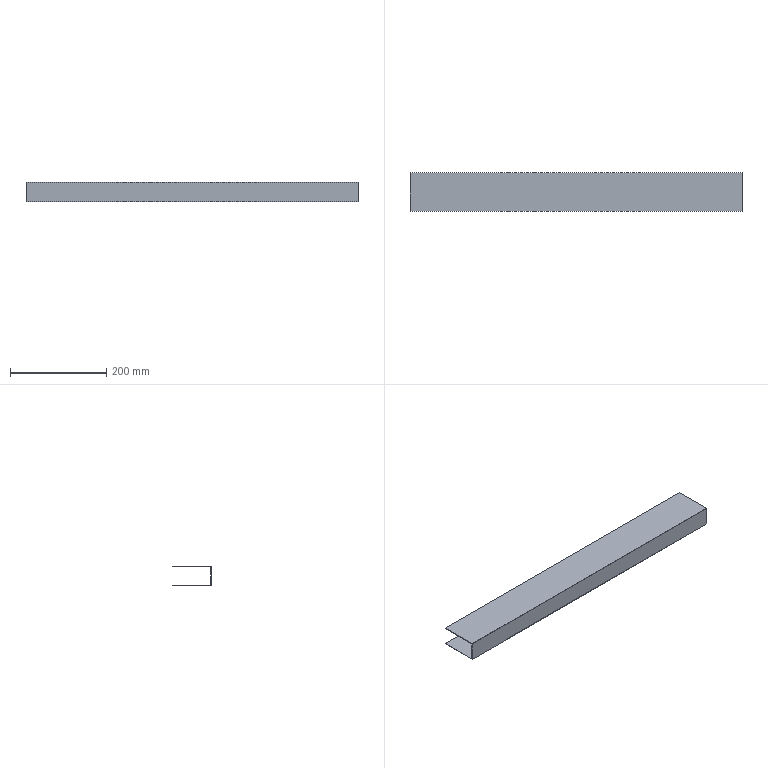Part | SolidWorks | features BaseBody 1 | 1 solid | 10 faces | box 690 x 80 x 40 mm | volume 136620 mm3 | plane 10
STEP:
#1=CARTESIAN_POINT('',(0.,1.,19.));
#2=VERTEX_POINT('',#1);
#3=CARTESIAN_POINT('',(0.,80.,19.));
#4=VERTEX_POINT('',#3);
#5=CARTESIAN_POINT('',(0.,0.,19.));
#6=DIRECTION('',(0.,1.,0.));
#7=VECTOR('',#6,1000.);
#8=LINE('',#5,#7);
#9=EDGE_CURVE('',#2,#4,#8,.T.);
#10=ORIENTED_EDGE('',*,*,#9,.F.);
#11=CARTESIAN_POINT('',(0.,1.,-19.));
#12=VERTEX_POINT('',#11);
#13=CARTESIAN_POINT('',(0.,1.,20.));
#14=DIRECTION('',(0.,0.,1.));
#15=VECTOR('',#14,1000.);
#16=LINE('',#13,#15);
#17=EDGE_CURVE('',#12,#2,#16,.T.);
#18=ORIENTED_EDGE('',*,*,#17,.F.);
#19=CARTESIAN_POINT('',(0.,80.,-19.));
#20=VERTEX_POINT('',#19);
#21=CARTESIAN_POINT('',(0.,0.,-19.));
#22=DIRECTION('',(0.,-1.,0.));
#23=VECTOR('',#22,1000.);
#24=LINE('',#21,#23);
#25=EDGE_CURVE('',#20,#12,#24,.T.);
#26=ORIENTED_EDGE('',*,*,#25,.F.);
#27=CARTESIAN_POINT('',(0.,80.,-20.));
#28=VERTEX_POINT('',#27);
#29=CARTESIAN_POINT('',(0.,80.,-19.));
#30=DIRECTION('',(0.,0.,-1.));
#31=VECTOR('',#30,1000.);
#32=LINE('',#29,#31);
#33=EDGE_CURVE('',#20,#28,#32,.T.);
#34=ORIENTED_EDGE('',*,*,#33,.T.);
#35=CARTESIAN_POINT('',(0.,0.,-20.));
#36=VERTEX_POINT('',#35);
#37=CARTESIAN_POINT('',(0.,0.,-20.));
#38=DIRECTION('',(0.,-1.,0.));
#39=VECTOR('',#38,1000.);
#40=LINE('',#37,#39);
#41=EDGE_CURVE('',#28,#36,#40,.T.);
#42=ORIENTED_EDGE('',*,*,#41,.T.);
#43=CARTESIAN_POINT('',(0.,0.,20.));
#44=VERTEX_POINT('',#43);
#45=CARTESIAN_POINT('',(0.,0.,20.));
#46=DIRECTION('',(0.,0.,1.));
#47=VECTOR('',#46,1000.);
#48=LINE('',#45,#47);
#49=EDGE_CURVE('',#36,#44,#48,.T.);
#50=ORIENTED_EDGE('',*,*,#49,.T.);
#51=CARTESIAN_POINT('',(0.,80.,20.));
#52=VERTEX_POINT('',#51);
#53=CARTESIAN_POINT('',(0.,0.,20.));
#54=DIRECTION('',(0.,1.,0.));
#55=VECTOR('',#54,1000.);
#56=LINE('',#53,#55);
#57=EDGE_CURVE('',#44,#52,#56,.T.);
#58=ORIENTED_EDGE('',*,*,#57,.T.);
#59=CARTESIAN_POINT('',(0.,80.,20.));
#60=DIRECTION('',(0.,0.,-1.));
#61=VECTOR('',#60,1000.);
#62=LINE('',#59,#61);
#63=EDGE_CURVE('',#52,#4,#62,.T.);
#64=ORIENTED_EDGE('',*,*,#63,.T.);
#65=EDGE_LOOP('',(#10,#18,#26,#34,#42,#50,#58,#64));
#66=FACE_OUTER_BOUND('',#65,.T.);
#67=CARTESIAN_POINT('',(0.,0.,0.));
#68=DIRECTION('',(-1.,0.,0.));
#69=DIRECTION('',(0.,0.,1.));
#70=AXIS2_PLACEMENT_3D('',#67,#68,#69);
#71=PLANE('',#70);
#72=ADVANCED_FACE('',(#66),#71,.T.);
#73=CARTESIAN_POINT('',(690.,1.,19.));
#74=VERTEX_POINT('',#73);
#75=CARTESIAN_POINT('',(690.,80.,19.));
#76=VERTEX_POINT('',#75);
#77=CARTESIAN_POINT('',(690.,0.,19.));
#78=DIRECTION('',(0.,1.,0.));
#79=VECTOR('',#78,1000.);
#80=LINE('',#77,#79);
#81=EDGE_CURVE('',#74,#76,#80,.T.);
#82=ORIENTED_EDGE('',*,*,#81,.T.);
#83=CARTESIAN_POINT('',(690.,80.,20.));
#84=VERTEX_POINT('',#83);
#85=CARTESIAN_POINT('',(690.,80.,20.));
#86=DIRECTION('',(0.,0.,-1.));
#87=VECTOR('',#86,1000.);
#88=LINE('',#85,#87);
#89=EDGE_CURVE('',#84,#76,#88,.T.);
#90=ORIENTED_EDGE('',*,*,#89,.F.);
#91=CARTESIAN_POINT('',(690.,0.,20.));
#92=VERTEX_POINT('',#91);
#93=CARTESIAN_POINT('',(690.,0.,20.));
#94=DIRECTION('',(0.,1.,0.));
#95=VECTOR('',#94,1000.);
#96=LINE('',#93,#95);
#97=EDGE_CURVE('',#92,#84,#96,.T.);
#98=ORIENTED_EDGE('',*,*,#97,.F.);
#99=CARTESIAN_POINT('',(690.,0.,-20.));
#100=VERTEX_POINT('',#99);
#101=CARTESIAN_POINT('',(690.,0.,20.));
#102=DIRECTION('',(0.,0.,1.));
#103=VECTOR('',#102,1000.);
#104=LINE('',#101,#103);
#105=EDGE_CURVE('',#100,#92,#104,.T.);
#106=ORIENTED_EDGE('',*,*,#105,.F.);
#107=CARTESIAN_POINT('',(690.,80.,-20.));
#108=VERTEX_POINT('',#107);
#109=CARTESIAN_POINT('',(690.,0.,-20.));
#110=DIRECTION('',(0.,-1.,0.));
#111=VECTOR('',#110,1000.);
#112=LINE('',#109,#111);
#113=EDGE_CURVE('',#108,#100,#112,.T.);
#114=ORIENTED_EDGE('',*,*,#113,.F.);
#115=CARTESIAN_POINT('',(690.,80.,-19.));
#116=VERTEX_POINT('',#115);
#117=CARTESIAN_POINT('',(690.,80.,-19.));
#118=DIRECTION('',(0.,0.,-1.));
#119=VECTOR('',#118,1000.);
#120=LINE('',#117,#119);
#121=EDGE_CURVE('',#116,#108,#120,.T.);
#122=ORIENTED_EDGE('',*,*,#121,.F.);
#123=CARTESIAN_POINT('',(690.,1.,-19.));
#124=VERTEX_POINT('',#123);
#125=CARTESIAN_POINT('',(690.,0.,-19.));
#126=DIRECTION('',(0.,-1.,0.));
#127=VECTOR('',#126,1000.);
#128=LINE('',#125,#127);
#129=EDGE_CURVE('',#116,#124,#128,.T.);
#130=ORIENTED_EDGE('',*,*,#129,.T.);
#131=CARTESIAN_POINT('',(690.,1.,20.));
#132=DIRECTION('',(0.,0.,1.));
#133=VECTOR('',#132,1000.);
#134=LINE('',#131,#133);
#135=EDGE_CURVE('',#124,#74,#134,.T.);
#136=ORIENTED_EDGE('',*,*,#135,.T.);
#137=EDGE_LOOP('',(#82,#90,#98,#106,#114,#122,#130,#136));
#138=FACE_OUTER_BOUND('',#137,.T.);
#139=CARTESIAN_POINT('',(690.,0.,0.));
#140=DIRECTION('',(-1.,0.,0.));
#141=DIRECTION('',(0.,0.,1.));
#142=AXIS2_PLACEMENT_3D('',#139,#140,#141);
#143=PLANE('',#142);
#144=ADVANCED_FACE('',(#138),#143,.F.);
#145=ORIENTED_EDGE('',*,*,#17,.T.);
#146=CARTESIAN_POINT('',(690.,1.,19.));
#147=DIRECTION('',(-1.,0.,0.));
#148=VECTOR('',#147,1000.);
#149=LINE('',#146,#148);
#150=EDGE_CURVE('',#74,#2,#149,.T.);
#151=ORIENTED_EDGE('',*,*,#150,.F.);
#152=ORIENTED_EDGE('',*,*,#135,.F.);
#153=CARTESIAN_POINT('',(690.,1.,-19.));
#154=DIRECTION('',(-1.,0.,0.));
#155=VECTOR('',#154,1000.);
#156=LINE('',#153,#155);
#157=EDGE_CURVE('',#124,#12,#156,.T.);
#158=ORIENTED_EDGE('',*,*,#157,.T.);
#159=EDGE_LOOP('',(#145,#151,#152,#158));
#160=FACE_OUTER_BOUND('',#159,.T.);
#161=CARTESIAN_POINT('',(690.,1.,20.));
#162=DIRECTION('',(0.,-1.,0.));
#163=DIRECTION('',(0.,0.,-1.));
#164=AXIS2_PLACEMENT_3D('',#161,#162,#163);
#165=PLANE('',#164);
#166=ADVANCED_FACE('',(#160),#165,.F.);
#167=ORIENTED_EDGE('',*,*,#25,.T.);
#168=ORIENTED_EDGE('',*,*,#157,.F.);
#169=ORIENTED_EDGE('',*,*,#129,.F.);
#170=CARTESIAN_POINT('',(690.,80.,-19.));
#171=DIRECTION('',(-1.,0.,0.));
#172=VECTOR('',#171,1000.);
#173=LINE('',#170,#172);
#174=EDGE_CURVE('',#116,#20,#173,.T.);
#175=ORIENTED_EDGE('',*,*,#174,.T.);
#176=EDGE_LOOP('',(#167,#168,#169,#175));
#177=FACE_OUTER_BOUND('',#176,.T.);
#178=CARTESIAN_POINT('',(690.,0.,-19.));
#179=DIRECTION('',(0.,0.,-1.));
#180=DIRECTION('',(0.,-1.,0.));
#181=AXIS2_PLACEMENT_3D('',#178,#179,#180);
#182=PLANE('',#181);
#183=ADVANCED_FACE('',(#177),#182,.F.);
#184=ORIENTED_EDGE('',*,*,#33,.F.);
#185=ORIENTED_EDGE('',*,*,#174,.F.);
#186=ORIENTED_EDGE('',*,*,#121,.T.);
#187=CARTESIAN_POINT('',(690.,80.,-20.));
#188=DIRECTION('',(-1.,0.,0.));
#189=VECTOR('',#188,1000.);
#190=LINE('',#187,#189);
#191=EDGE_CURVE('',#108,#28,#190,.T.);
#192=ORIENTED_EDGE('',*,*,#191,.T.);
#193=EDGE_LOOP('',(#184,#185,#186,#192));
#194=FACE_OUTER_BOUND('',#193,.T.);
#195=CARTESIAN_POINT('',(690.,80.,-19.));
#196=DIRECTION('',(0.,1.,0.));
#197=DIRECTION('',(1.,0.,0.));
#198=AXIS2_PLACEMENT_3D('',#195,#196,#197);
#199=PLANE('',#198);
#200=ADVANCED_FACE('',(#194),#199,.T.);
#201=ORIENTED_EDGE('',*,*,#41,.F.);
#202=ORIENTED_EDGE('',*,*,#191,.F.);
#203=ORIENTED_EDGE('',*,*,#113,.T.);
#204=CARTESIAN_POINT('',(690.,0.,-20.));
#205=DIRECTION('',(-1.,0.,0.));
#206=VECTOR('',#205,1000.);
#207=LINE('',#204,#206);
#208=EDGE_CURVE('',#100,#36,#207,.T.);
#209=ORIENTED_EDGE('',*,*,#208,.T.);
#210=EDGE_LOOP('',(#201,#202,#203,#209));
#211=FACE_OUTER_BOUND('',#210,.T.);
#212=CARTESIAN_POINT('',(690.,0.,-20.));
#213=DIRECTION('',(0.,0.,-1.));
#214=DIRECTION('',(0.,-1.,0.));
#215=AXIS2_PLACEMENT_3D('',#212,#213,#214);
#216=PLANE('',#215);
#217=ADVANCED_FACE('',(#211),#216,.T.);
#218=ORIENTED_EDGE('',*,*,#49,.F.);
#219=ORIENTED_EDGE('',*,*,#208,.F.);
#220=ORIENTED_EDGE('',*,*,#105,.T.);
#221=CARTESIAN_POINT('',(690.,0.,20.));
#222=DIRECTION('',(-1.,0.,0.));
#223=VECTOR('',#222,1000.);
#224=LINE('',#221,#223);
#225=EDGE_CURVE('',#92,#44,#224,.T.);
#226=ORIENTED_EDGE('',*,*,#225,.T.);
#227=EDGE_LOOP('',(#218,#219,#220,#226));
#228=FACE_OUTER_BOUND('',#227,.T.);
#229=CARTESIAN_POINT('',(690.,0.,20.));
#230=DIRECTION('',(0.,-1.,0.));
#231=DIRECTION('',(0.,0.,-1.));
#232=AXIS2_PLACEMENT_3D('',#229,#230,#231);
#233=PLANE('',#232);
#234=ADVANCED_FACE('',(#228),#233,.T.);
#235=ORIENTED_EDGE('',*,*,#57,.F.);
#236=ORIENTED_EDGE('',*,*,#225,.F.);
#237=ORIENTED_EDGE('',*,*,#97,.T.);
#238=CARTESIAN_POINT('',(690.,80.,20.));
#239=DIRECTION('',(-1.,0.,0.));
#240=VECTOR('',#239,1000.);
#241=LINE('',#238,#240);
#242=EDGE_CURVE('',#84,#52,#241,.T.);
#243=ORIENTED_EDGE('',*,*,#242,.T.);
#244=EDGE_LOOP('',(#235,#236,#237,#243));
#245=FACE_OUTER_BOUND('',#244,.T.);
#246=CARTESIAN_POINT('',(690.,0.,20.));
#247=DIRECTION('',(0.,0.,1.));
#248=DIRECTION('',(0.,-1.,0.));
#249=AXIS2_PLACEMENT_3D('',#246,#247,#248);
#250=PLANE('',#249);
#251=ADVANCED_FACE('',(#245),#250,.T.);
#252=ORIENTED_EDGE('',*,*,#63,.F.);
#253=ORIENTED_EDGE('',*,*,#242,.F.);
#254=ORIENTED_EDGE('',*,*,#89,.T.);
#255=CARTESIAN_POINT('',(690.,80.,19.));
#256=DIRECTION('',(-1.,0.,0.));
#257=VECTOR('',#256,1000.);
#258=LINE('',#255,#257);
#259=EDGE_CURVE('',#76,#4,#258,.T.);
#260=ORIENTED_EDGE('',*,*,#259,.T.);
#261=EDGE_LOOP('',(#252,#253,#254,#260));
#262=FACE_OUTER_BOUND('',#261,.T.);
#263=CARTESIAN_POINT('',(690.,80.,20.));
#264=DIRECTION('',(0.,1.,0.));
#265=DIRECTION('',(1.,0.,0.));
#266=AXIS2_PLACEMENT_3D('',#263,#264,#265);
#267=PLANE('',#266);
#268=ADVANCED_FACE('',(#262),#267,.T.);
#269=ORIENTED_EDGE('',*,*,#9,.T.);
#270=ORIENTED_EDGE('',*,*,#259,.F.);
#271=ORIENTED_EDGE('',*,*,#81,.F.);
#272=ORIENTED_EDGE('',*,*,#150,.T.);
#273=EDGE_LOOP('',(#269,#270,#271,#272));
#274=FACE_OUTER_BOUND('',#273,.T.);
#275=CARTESIAN_POINT('',(690.,0.,19.));
#276=DIRECTION('',(0.,0.,1.));
#277=DIRECTION('',(0.,-1.,0.));
#278=AXIS2_PLACEMENT_3D('',#275,#276,#277);
#279=PLANE('',#278);
#280=ADVANCED_FACE('',(#274),#279,.F.);
#281=CLOSED_SHELL('',(#72,#144,#166,#183,#200,#217,#234,#251,#268,#280));
#282=MANIFOLD_SOLID_BREP('',#281);
#283=CARTESIAN_POINT('',(0.,0.,0.));
#284=DIRECTION('',(0.,0.,1.));
#285=DIRECTION('',(1.,0.,0.));
#286=AXIS2_PLACEMENT_3D('',#283,#284,#285);
#287=(LENGTH_UNIT()NAMED_UNIT(*)SI_UNIT(.MILLI.,.METRE.));
#288=UNCERTAINTY_MEASURE_WITH_UNIT(LENGTH_MEASURE(0.00001),#287,'','');
#289=(NAMED_UNIT(*)PLANE_ANGLE_UNIT()SI_UNIT($,.RADIAN.));
#290=(NAMED_UNIT(*)SI_UNIT($,.STERADIAN.)SOLID_ANGLE_UNIT());
#291=(GEOMETRIC_REPRESENTATION_CONTEXT(3)GLOBAL_UNCERTAINTY_ASSIGNED_CONTEXT((#288))GLOBAL_UNIT_ASSIGNED_CONTEXT((#287,#289,#290))REPRESENTATION_CONTEXT('',''));
#292=ADVANCED_BREP_SHAPE_REPRESENTATION('',(#282,#286),#291);